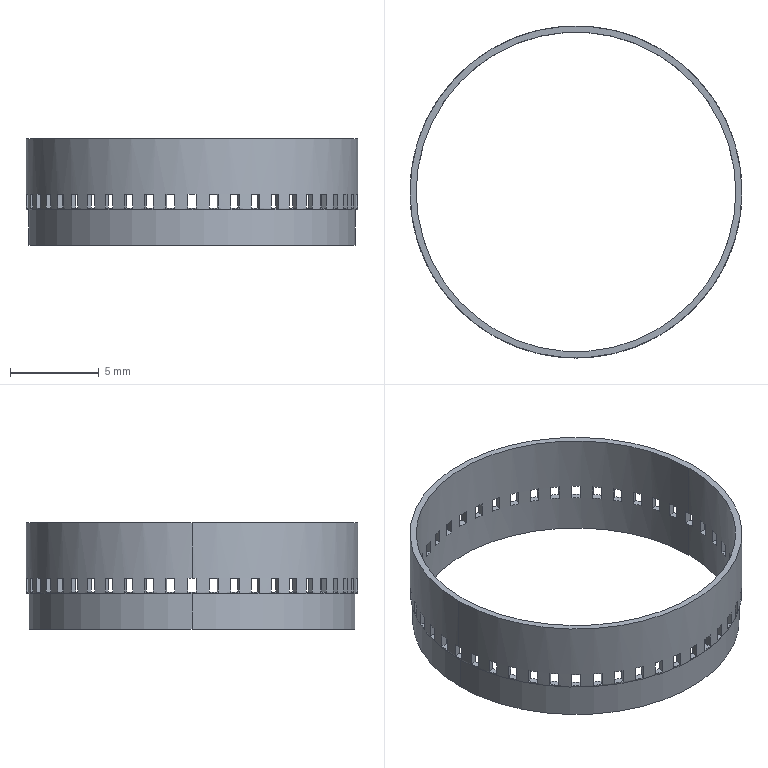Part | SolidWorks | features ICE 3, CirPattern 1, Extrusion 1 | 1 solid | 201 faces | box 18.7 x 18.7 x 6 mm | volume 97.096 mm3 | plane 195 | cylinder 6 | commonest cylinder face diameters 18 x2 18.4 x2 18.7 x2